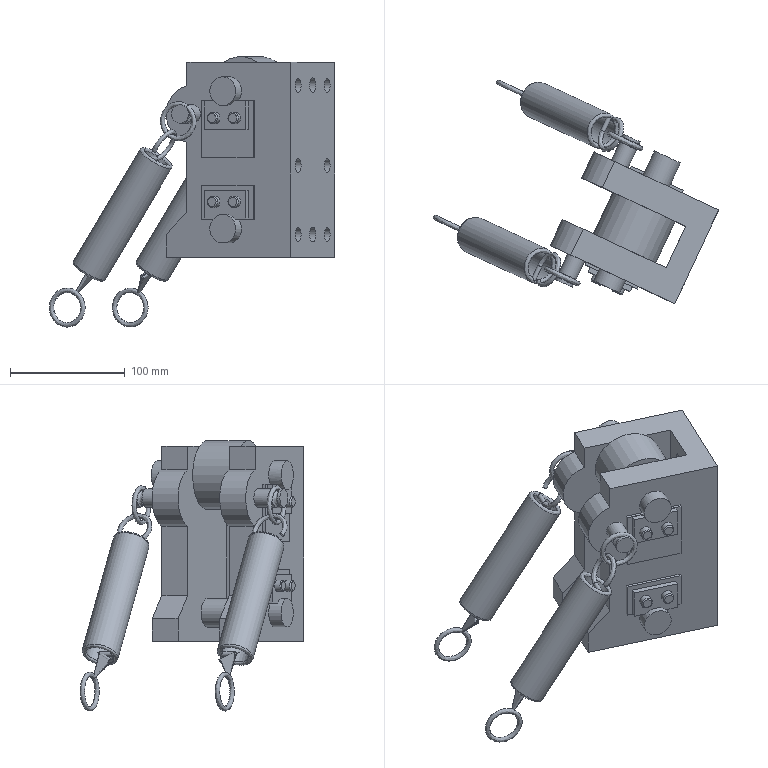Part | NX | features .2 ( *SOL5 - WSP HPSL15-R -  ) 2 | 1 solid | 137 faces | box 248.675 x 195.042 x 235.732 mm | volume 1315032 mm3 | plane 82 | cylinder 32 | spline 15 | cone 8 | commonest cylinder face diameters 12 x6 25 x5 4 x4 10 x4 16 x4 13 x2